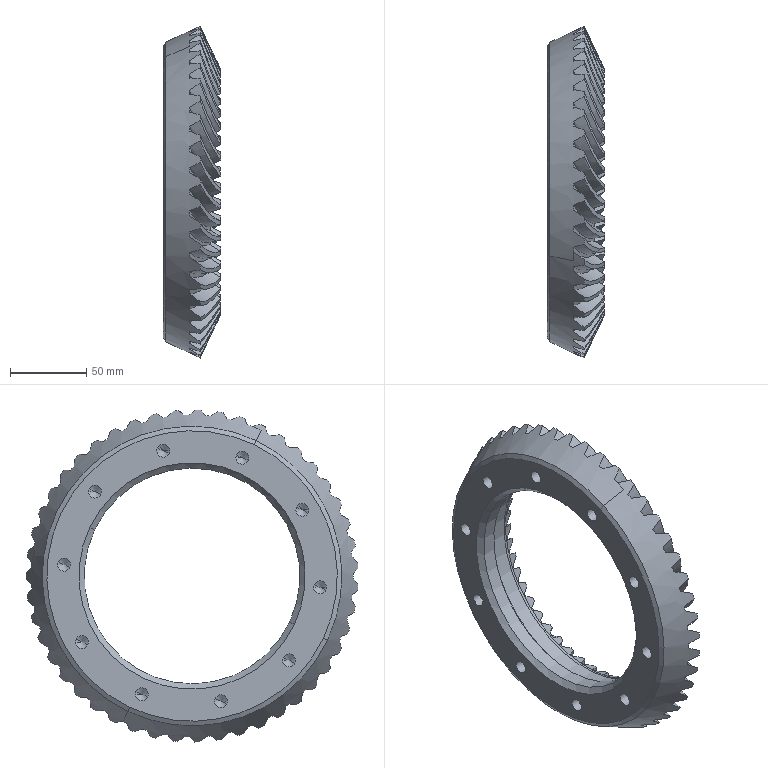Part | NX | features BREP 1 | 1 solid | 251 faces | box 37.698 x 217.333 x 217.419 mm | volume 451944 mm3 | cone 129 | spline 94 | cylinder 24 | torus 2 | plane 2 | commonest cylinder face diameters 8.433 x20 141.26 x2 151.25 x2